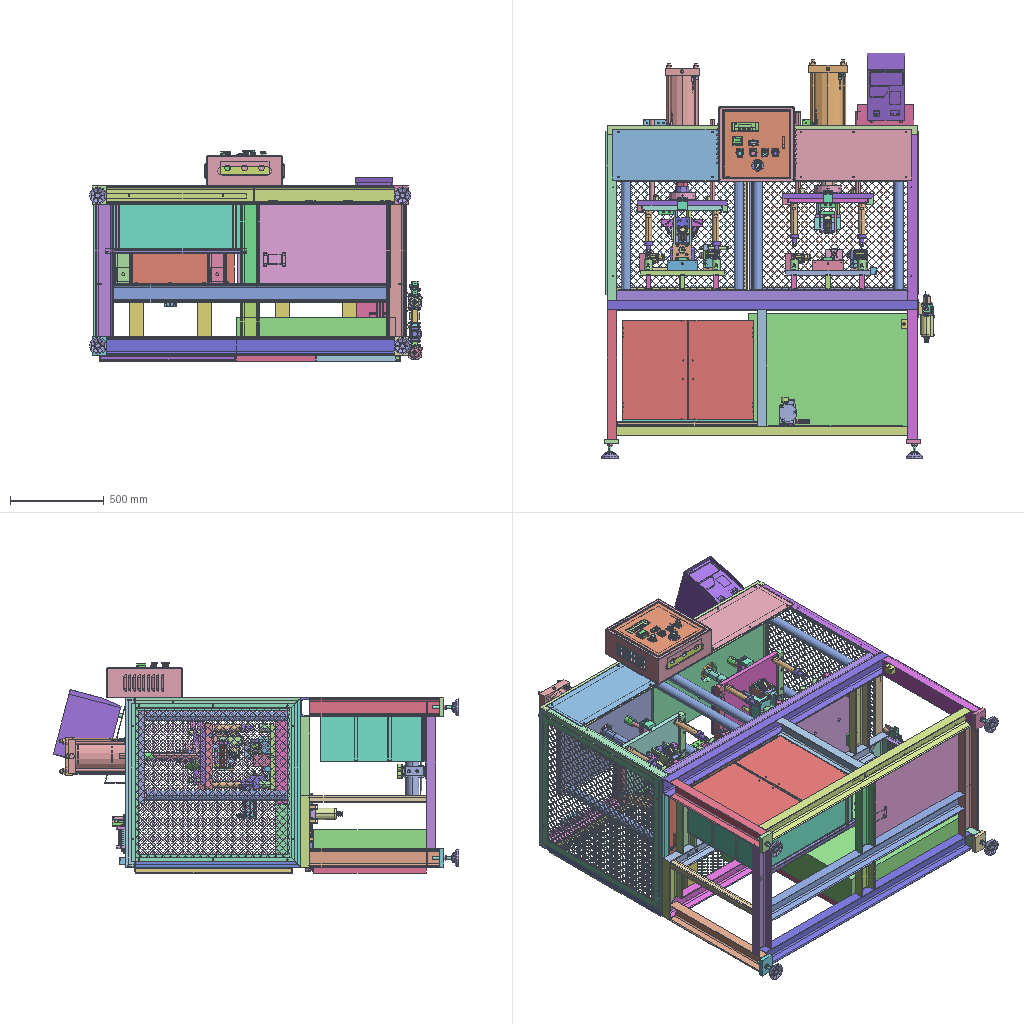Assembly | STEP file | 178 different items | 377 placed | box 1770 x 2157 x 1125 mm
Parts list (item | name | quantity | parent item | size | volume):
1 | CDS1FN160-250-A54Z_CS1-Body-1 | x1 | in CDS1FN160-250-A54Z | 182 x 182 x 425 mm | 4151915 mm3
2 | CDS1FN160-250-A54Z_CS1-Rod | x2 | in CDS1FN160-250-A54Z | 160 x 160 x 425.5 mm | 614336 mm3
3 | CDS1FN160-250-A54Z_CS1-Flange | x1 | in CDS1FN160-250-A54Z | 275 x 180 x 20 mm | 823998 mm3
4 | CDS1FN160-250-A54Z_A5_A6_F5_J5_ForLargeBore | x2 | in CDS1FN160-250-A54Z | 32 x 26 x 89 mm | 7994 mm3
5 | CDS1FN180-250-A54Z_CS1-Rod | x2 | in CDS1FN180-250-A54Z | 180 x 180 x 445 mm | 804374 mm3
6 | CDS1FN180-250-A54Z_CS1-Body-1 | x1 | in CDS1FN180-250-A54Z | 204 x 204 x 444 mm | 5555129 mm3
7 | CDS1FN180-250-A54Z_CS1-Flange | x1 | in CDS1FN180-250-A54Z | 320 x 200 x 25 mm | 1269642 mm3
8 | CDS1FN180-250-A54Z_A5_A6_F5_J5_ForLargeBore | x2 | in CDS1FN180-250-A54Z | 34 x 28 x 89 mm | 8233 mm3
9 | NT-16_CS1-RodEndNut | x1 | in NT-16 | 55 x 63.509 x 21 mm | 33434 mm3
10 | NT-18_Nuts | x1 | in NT-18 | 60.016 x 69.3 x 23 mm | 42288 mm3
11 | CQ2B40-30D_CQ2Tube | x4 | in CQ2B40-30D, CQ2B40-30D-1, CQ2B40-30D-2, CQ2B40-30D-3 | 52 x 57 x 59.5 mm | 79624 mm3
12 | CQ2B40-30D_CQ22031Rods | x4 | in CQ2B40-30D, CQ2B40-30D-1, CQ2B40-30D-2, CQ2B40-30D-3 | 40 x 40 x 54.25 mm | 15444 mm3
13 | CQ2B40-30D_CQ2 SnapRing | x4 | in CQ2B40-30D, CQ2B40-30D-1, CQ2B40-30D-2, CQ2B40-30D-3 | 44.5 x 43.888 x 7 mm | 5046 mm3
14 | HANYOUNG CR-253 5A | x2 | in Assy Hanyoung CR-253, panel box 500 x 600 x 200 | 32.5 x 45.5 x 64.5 mm | 42497 mm3
15 | Switch CR-253 | x1 | in Assy Hanyoung CR-253 | 24 x 35.897 x 23 mm | 7467 mm3
16 | B18.6.7M - M3 x 0.5 x 5 Type I Cross Recessed PHMS --5N | x8 | in Assy Hanyoung CR-253, Assy H7EC | 7.373 x 5.6 x 5.6 mm | 81.485 mm3
17 | OMRON H7EC | x1 | in Assy H7EC | 47.6 x 23.8 x 55.5 mm | 8164 mm3
18 | B18.6.7M - M4 x 0.7 x 5 Type I Cross Recessed PHMS --5N | x4 | in Assy H7EC | 8.067 x 8 x 8 mm | 178.262 mm3
19 | Cover | x1 | in Assy H7EC | 48 x 35 x 26.5 mm | 5852 mm3
20 | Karet | x1 | in Assy H7EC | 50 x 27 x 2.5 mm | 725.773 mm3
21 | Omron | x1 | in COUNTER OMRON | 109 x 47.8 x 53.73 mm | 203116 mm3
22 | panel body | x1 | in panel box 500 x 600 x 200 | 424 x 400 x 160 mm | 948430 mm3
23 | panel body dalam | x1 | in panel box 500 x 600 x 200 | 300 x 300 x 10 mm | 177458 mm3
24 | tutup bawah | x1 | in panel box 500 x 600 x 200 | 260 x 1.8 x 70 mm | 28943 mm3
25 | panel body depan | x1 | in panel box 500 x 600 x 200 | 352 x 381.4 x 22.754 mm | 281354 mm3
26 | Vexta Operation Unit OP200A | x1 | in panel box 500 x 600 x 200 | 142 x 48 x 17.4 mm | 105973 mm3
27 | Emergency hanyoung | x1 | in panel box 500 x 600 x 200 | 39.095 x 47.049 x 74 mm | 39082 mm3
28 | push_lamp1 | x1 | in panel box 500 x 600 x 200 | 36 x 54.3 x 68.1 mm | 76407 mm3
29 | Fuji Electric AR9T511-M | x1 | in panel box 500 x 600 x 200 | 30 x 39.5 x 78 mm | 61141 mm3
30 | Emergency Label | x1 | in panel box 500 x 600 x 200 | 64 x 1 x 64 mm | 2571 mm3
31 | Legend Standby | x4 | in panel box 500 x 600 x 200 | 41.068 x 43.269 x 1.43 mm | 1005 mm3
32 | CQ2A50-125DC-R06US_AS3054 Body | x2 | in CQ2A50-125DC-R06US_AS3054, CQ2A50-125DC-R06US_AS3054-1 | 34.45 x 40.4 x 19.63 mm | 8086 mm3
33 | CQ2A50-125DC-R06US_CQ2Tube | x1 | in CQ2A50-125DC-R06US | 64 x 71 x 180.5 mm | 380542 mm3
34 | CQ2A50-125DC-R06US_CQ22031Rods | x1 | in CQ2A50-125DC-R06US | 50 x 50 x 173.25 mm | 61293 mm3
35 | CQ2A50-125DC-R06US_CQ2 SnapRing | x1 | in CQ2A50-125DC-R06US | 55 x 54.243 x 13.3 mm | 12652 mm3
36 | AC10B-M5_AC3011A Spacer Interface(1) | x1 | in AC10B-M5_AC3011A Spacer(100T) | 6 x 25.75 x 33 mm | 2218 mm3
37 | AC10B-M5_AC3011A Spacer Front Plate(1) | x1 | in AC10B-M5_AC3011A Spacer(100T) | 13.502 x 24.5 x 7.058 mm | 480.167 mm3
38 | AC10B-M5_AC3011A AF Bowl(10)-1 | x1 | in AC10B-M5_AC3011A AF Bowl Assy(10) | 26.2 x 41.1 x 26.2 mm | 3344 mm3
39 | AC10B-M5_AC3011A AF Drain(10)-1 | x1 | in AC10B-M5_AC3011A AF Bowl Assy(10) | 11.5 x 8.4 x 11.5 mm | 268.613 mm3
40 | AC10B-M5_AC3011A AF Body(10)-1 | x1 | in AC10B-M5 | 25 x 17.5 x 25 mm | 8195 mm3
41 | AC10B-M5_AC3011A AR Body(10)-1 | x1 | in AC10B-M5 | 25 x 58 x 25 mm | 17859 mm3
42 | AC10B-M5_AC3011A Plug(00) | x2 | in AC10B-M5 | 6.85 x 8.115 x 8.115 mm | 313.171 mm3
43 | Cosmo LS-1862 | x1 | in 43 | 198 x 303.553 x 384.993 mm | 18480942 mm3
44 | SS5V1-16S3AD-08B-N1_CAInput Side End Plate | x1 | in SS5V1-16S3AD-08B-N1_EX120 Connector Block | 30 x 67.2 x 95.55 mm | 93320 mm3
45 | SS5V1-16S3AD-08B-N1_Rail Clamp | x2 | in SS5V1-16S3AD-08B-N1_EX120 Connector Block, SS5V1-16S3AD-08B-N1_CAExhaust Side | 11 x 10 x 87 mm | 2335 mm3
46 | SS5V1-16S3AD-08B-N1_Exhaust Cap | x2 | in SS5V1-16S3AD-08B-N1_EX120 Connector Block, SS5V1-16S3AD-08B-N1_CAExhaust Side | 16.5 x 8.5 x 63 mm | 8670 mm3
47 | SS5V1-16S3AD-08B-N1_SV Fittings | x4 | in SS5V1-16S3AD-08B-N1_EX120 Connector Block, SS5V1-16S3AD-08B-N1_CAExhaust Side | 14 x 14 x 19.5 mm | 1887 mm3
48 | SS5V1-16S3AD-08B-N1_EX120 Adapter | x1 | in SS5V1-16S3AD-08B-N1_EX120 Connector Block | 68.5 x 61 x 26.75 mm | 64315 mm3
49 | SS5V1-16S3AD-08B-N1_EX120 SI Unit | x1 | in SS5V1-16S3AD-08B-N1_EX120 Connector Block | 64 x 61 x 28.8 mm | 102624 mm3
50 | SS5V1-16S3AD-08B-N1_Valve Base | x8 | in SS5V1-16S3AD-08B-N1_Base, SS5V1-16S3AD-08B-N1_Base-1, SS5V1-16S3AD-08B-N1_Base-2, SS5V1-16S3AD-08B-N1_Base-3, SS5V1-16S3AD-08B-N1_Base-4, SS5V1-16S3AD-08B-N1_Base-5, SS5V1-16S3AD-08B-N1_Base-6, SS5V1-16S3AD-08B-N1_Base-7 | 10.5 x 34 x 95.55 mm | 27614 mm3
51 | SS5V1-16S3AD-08B-N1_VV5Q Fittings | x16 | in SS5V1-16S3AD-08B-N1_Base, SS5V1-16S3AD-08B-N1_Base-1, SS5V1-16S3AD-08B-N1_Base-2, SS5V1-16S3AD-08B-N1_Base-3, SS5V1-16S3AD-08B-N1_Base-4, SS5V1-16S3AD-08B-N1_Base-5, SS5V1-16S3AD-08B-N1_Base-6, SS5V1-16S3AD-08B-N1_Base-7 | 10 x 10 x 16 mm | 989.757 mm3
52 | SS5V1-16S3AD-08B-N1_CAD Side End Plate | x1 | in SS5V1-16S3AD-08B-N1_CAExhaust Side | 30.5 x 38.5 x 95.55 mm | 62940 mm3
53 | SS5V1-16S3AD-08B-N1_AXT100-DR | x1 | in SS5V1-16S3AD-08B-N1 | 35 x 7.5 x 210.5 mm | 13884 mm3
54 | VBA22A-03GN_AN6009 Silencer | x1 | in VBA22A-03GN_AN6009 | 25.403 x 84 x 25 mm | 9196 mm3
55 | VBA22A-03GN_VBA20A Body | x1 | in VBA22A-03GN | 300 x 127.5 x 92.8 mm | 1446394 mm3
56 | VBA22A-03GN_G36-10-N01 | x2 | in VBA22A-03GN | 37 x 41.5 x 37 mm | 27826 mm3
57 | VBA22A-03GN_VBA20A Bracket | x1 | in VBA22A-03GN | 118 x 11 x 73 mm | 25260 mm3
58 | AC40-04-KSTV-38JNR_AC3009A Spacer Interface | x6 | in AC40-04-KSTV-38JNR_AC3009A Spacer(400T-R), AC40-04-KSTV-38JNR_AC3009A Spacer(400-R), AC40-04-KSTV-38JNR_AC3009A Spacer(400T-R)-1, AC40-04-KSTV-38JNR_AC3009A Spacer(400-R)-1, AC40-04-KSTV-38JNR_AC3009A Spacer(400T-R)-2, AC40-04-KSTV-38JNR_AC3009A Spacer(400T-R)-3 | 9 x 56.65 x 65 mm | 9428 mm3
59 | AC40-04-KSTV-38JNR_AC3009A Spacer Rear Plate(4T) | x4 | in AC40-04-KSTV-38JNR_AC3009A Spacer(400T-R), AC40-04-KSTV-38JNR_AC3009A Spacer(400T-R)-1, AC40-04-KSTV-38JNR_AC3009A Spacer(400T-R)-2, AC40-04-KSTV-38JNR_AC3009A Spacer(400T-R)-3 | 26 x 96 x 34.173 mm | 17760 mm3
60 | AC40-04-KSTV-38JNR_AC3009A Spacer Front Plate | x6 | in AC40-04-KSTV-38JNR_AC3009A Spacer(400T-R), AC40-04-KSTV-38JNR_AC3009A Spacer(400-R), AC40-04-KSTV-38JNR_AC3009A Spacer(400T-R)-1, AC40-04-KSTV-38JNR_AC3009A Spacer(400-R)-1, AC40-04-KSTV-38JNR_AC3009A Spacer(400T-R)-2, AC40-04-KSTV-38JNR_AC3009A Spacer(400T-R)-3 | 18.505 x 54.2 x 10.913 mm | 2347 mm3
61 | AC40-04-KSTV-38JNR_AC3009A Spacer Rear Plate(4) | x2 | in AC40-04-KSTV-38JNR_AC3009A Spacer(400-R), AC40-04-KSTV-38JNR_AC3009A Spacer(400-R)-1 | 18.951 x 54 x 7.773 mm | 1709 mm3
62 | AC40-04-KSTV-38JNR_AC3009A AF Bowl-2 | x1 | in AC40-04-KSTV-38JNR_AC3009A AF Bowl Assy | 61.5 x 121.9 x 71.711 mm | 50188 mm3
63 | AC40-04-KSTV-38JNR_AC3009A AF Drain-2 | x1 | in AC40-04-KSTV-38JNR_AC3009A AF Bowl Assy | 19.63 x 18.1 x 17 mm | 2625 mm3
64 | AC40-04-KSTV-38JNR_AC3009A AL Bowl-2 | x1 | in AC40-04-KSTV-38JNR_AC3009A AL Bowl Assy | 61.5 x 121.9 x 71.711 mm | 50188 mm3
65 | AC40-04-KSTV-38JNR_AC3009A AL Drain-2 | x1 | in AC40-04-KSTV-38JNR_AC3009A AL Bowl Assy | 28 x 24.1 x 28 mm | 7214 mm3
66 | AC40-04-KSTV-38JNR_AC3009A VHS Body-1 | x1 | in AC40-04-KSTV-38JNR_AC3009A VHS | 70 x 60.6 x 58 mm | 70876 mm3
67 | AC40-04-KSTV-38JNR_AC3009A VHS Handle | x1 | in AC40-04-KSTV-38JNR_AC3009A VHS | 63 x 46.4 x 58 mm | 68850 mm3
68 | AC40-04-KSTV-38JNR_AC3009A AR Body-1 | x1 | in AC40-04-KSTV-38JNR | 70 x 128 x 57.6 mm | 240174 mm3
69 | AC40-04-KSTV-38JNR_AC3009A T Interface-1 | x1 | in AC40-04-KSTV-38JNR | 24 x 62 x 36 mm | 21819 mm3
70 | AC40-04-KSTV-38JNR_AC3009A AF Body-1 | x1 | in AC40-04-KSTV-38JNR | 70 x 52 x 70 mm | 171815 mm3
71 | AC40-04-KSTV-38JNR_AC3009A Switch | x1 | in AC40-04-KSTV-38JNR | 15 x 111 x 36 mm | 31675 mm3
72 | AC40-04-KSTV-38JNR_AC3009A AKM Body | x1 | in AC40-04-KSTV-38JNR | 70 x 42 x 54 mm | 78893 mm3
73 | AC40-04-KSTV-38JNR_AC3009A AL Body-1 | x1 | in AC40-04-KSTV-38JNR | 70 x 74 x 70 mm | 184515 mm3
74 | AC40-04-KSTV-38JNR_AC3009A Gauge-2 | x1 | in AC40-04-KSTV-38JNR | 28 x 28 x 5 mm | 3081 mm3
75 | AC40-04-KSTV-38JNR_AC3009A Plug | x1 | in AC40-04-KSTV-38JNR | 10.8 x 13.845 x 13.845 mm | 1426 mm3
76 | OP10-001_base frame(Default_As Machined_) | x1 | - | 1680 x 792 x 900 mm | 25499684 mm3
77 | OP10-002_upper frame(Default_As Machined_) | x1 | - | 1650 x 1042 x 900 mm | 8540478 mm3
78 | OP10-003_front cover (R) | x1 | - | 620 x 5 x 270 mm | 835492 mm3
79 | OP10-004_front cover (L) | x1 | - | 560 x 5 x 270 mm | 754995 mm3
80 | OP10-005_side cover | x2 | - | - | 1174721 mm3
81 | OP10-006_rear cover (R) | x1 | - | - | 1354437 mm3
82 | OP10-007_rear cover (L) | x1 | - | - | 1150842 mm3
83 | OP10-009_shelf(Default_As Machined_) | x1 | - | 750 x 565 x 320 mm | 3649347 mm3
84 | OP10-010_junction block (A) | x2 | - | 220 x 35 x 35 mm | 246704 mm3
85 | OP10-011_junction block (B) | x1 | - | 190 x 35 x 35 mm | 212721 mm3
86 | OP10-012_junction block (C) | x1 | - | 130 x 35 x 35 mm | 144755 mm3
87 | OP10-013_junction block (D) | x1 | - | 50 x 35 x 35 mm | 54198 mm3
88 | OP10-014_lower plate (R) | x1 | - | 830 x 30 x 500 mm | 12317635 mm3
89 | OP10-015_upper plate (R) | x1 | - | 830 x 30 x 500 mm | 11965726 mm3
90 | OP10-016_lower plate (L)  | x1 | - | 680 x 30 x 500 mm | 10067635 mm3
91 | OP10-017_upper plate (L) | x1 | - | 680 x 30 x 500 mm | 9842603 mm3
92 | OP10-018_base rib (A) | x2 | - | 25 x 75 x 500 mm | 930693 mm3
93 | OP10-019_base rib (B) | x4 | - | 25 x 75 x 500 mm | 929254 mm3
94 | OP10-020_central plate | x2 | - | 480 x 25 x 300 mm | 3542194 mm3
95 | OP10-021_guide(1) | x2 | - | 35 x 35 x 350 mm | 297564 mm3
96 | OP10-022_guide(2) | x2 | - | 35 x 35 x 350 mm | 297564 mm3
97 | OP10-023_clamp | x8 | - | 35 x 12 x 19 mm | 6394 mm3
98 | OP10-024_fix-pin | x4 | - | 25 x 72 x 25 mm | 20386 mm3
99 | OP10-025_stopper base | x2 | - | 65 x 28 x 50 mm | 72632 mm3
100 | OP10-026_stopper plate | x2 | - | 65 x 20 x 50 mm | 54932 mm3
101 | OP10-027_cylinder connector (R) | x1 | - | 70 x 85 x 85 mm | 228647 mm3
102 | OP10-028_cylinder connector (L) | x1 | - | 75 x 85 x 85 mm | 251301 mm3
103 | OP10-029_setting flange | x2 | - | 139.943 x 36 x 140 mm | 309110 mm3
104 | OP10-030_plate | x2 | - | 140 x 5 x 140 mm | 72351 mm3
105 | OP10-031_guide base | x4 | - | 250 x 22 x 75 mm | 400090 mm3
106 | OP10-032_collar | x8 | - | 30 x 13 x 30 mm | 7922 mm3
107 | OP10-033_setup guide  | x4 | - | 25 x 100 x 300 mm | 745616 mm3
108 | OP10-034_shelf-door | x2 | - | 530 x 5 x 345 mm | 913394 mm3
109 | OP10-101_base plate lower (R) | x1 | - | 450 x 25 x 350 mm | 3845451 mm3
110 | OP10-102_base plate lower (L) | x1 | - | 450 x 25 x 350 mm | 3834229 mm3
111 | OP10-104_upper base plate (R) | x1 | - | 430 x 25 x 350 mm | 3618986 mm3
112 | OP10-105_upper base plate (L)  | x1 | - | 430 x 25 x 350 mm | 3617980 mm3
113 | OP10-106_guide post | x8 | - | 35 x 178 x 35 mm | 152676 mm3
114 | OP10-107_guide-pin | x8 | - | 44 x 44 x 91 mm | 50039 mm3
115 | OP10-108_guide catch | x8 | - | 44 x 44 x 84 mm | 74087 mm3
116 | OP10-109_base block (lower)-R | x1 | - | 160 x 50 x 160 mm | 1246879 mm3
117 | OP10-111_base block (lower)-L  | x1 | - | 160 x 50 x 160 mm | 1248387 mm3
118 | OP10-113_round-pin | x2 | - | 12 x 12 x 27.5 mm | 2777 mm3
119 | OP10-114_dia-pin | x2 | - | 12 x 12 x 27.5 mm | 2777 mm3
120 | OP10-116_work-guide | x2 | - | 14 x 20 x 70 mm | 17393 mm3
121 | OP10-118_cylinder base (1) | x3 | - | 86 x 13 x 69 mm | 65313 mm3
122 | OP10-119_cylinder stand (1) -R | x1 | - | 86 x 13 x 94 mm | 86706 mm3
123 | OP10-120_cylinder stand (1) -L | x1 | - | 86 x 13 x 94 mm | 86098 mm3
124 | OP10-121_cylinder stand (2) -R | x1 | - | 86 x 13 x 98 mm | 98029 mm3
125 | OP10-122_rib plate | x6 | - | 13 x 50 x 56 mm | 32347 mm3
126 | OP10-123_seal rod | x4 | - | 31 x 38 x 31 mm | 15633 mm3
127 | OP10-124_seal pad | x4 | - | 31 x 10 x 31 mm | 7003 mm3
128 | OP10-125_seal rod dia7 | x1 | - | 20 x 38 x 20 mm | 6478 mm3
129 | OP10-126_seal pad dia7 | x1 | - | 14 x 10 x 14 mm | 1539 mm3
130 | OP10-127_cylinder base M6 | x1 | - | 30 x 30 x 80 mm | 45481 mm3
131 | OP10-128_seal head M6 | x1 | - | 16 x 18 x 16 mm | 2771 mm3
132 | OP10-129_seal pad M6 | x1 | - | 11 x 10 x 11 mm | 950.332 mm3
133 | OP10-130_cylinder base (2)-L | x1 | - | 128 x 20 x 70 mm | 155973 mm3
134 | OP10-131_cylinder stand (2) -L | x1 | - | 100 x 20 x 125 mm | 216562 mm3
135 | OP10-132_side plate (2)-L | x2 | - | 100 x 14 x 70 mm | 92004 mm3
136 | OP10-133_seal rod camshaft | x1 | - | 31 x 40 x 31 mm | 16299 mm3
137 | OP10-134_cylinder stand (3) | x2 | - | 88 x 38 x 60 mm | 176864 mm3
138 | OP10-135_junction block (E) | x1 | - | 170 x 35 x 35 mm | 190983 mm3
139 | OP10-136_junction block (F) | x1 | - | 200 x 35 x 35 mm | 224966 mm3
140 | OP10-137_base block (upper)-R | x1 | - | 130 x 20 x 130 mm | 318432 mm3
141 | OP10-139_base plate (F)-R | x1 | - | 72 x 14 x 100 mm | 94613 mm3
142 | OP10-140_side plate (F)-R | x2 | - | 10 x 48 x 110 mm | 45630 mm3
143 | OP10-141_inclined plate (F) | x2 | - | 72 x 14 x 58 mm | 45441 mm3
144 | OP10-142_seal rod plug | x2 | - | 22 x 38 x 22 mm | 7650 mm3
145 | OP10-143_seal pad plug | x2 | - | 16 x 10 x 16 mm | 2011 mm3
146 | OP10-144_upper seal block | x1 | - | 130 x 59.5 x 135 mm | 671635 mm3
147 | OP10-146_seal side plate (1) | x1 | - | 44 x 10 x 72 mm | 28330 mm3
148 | OP10-147_seal side plate (2) | x1 | - | 22 x 12 x 44 mm | 7394 mm3
149 | OP10-148_seal block | x1 | - | 25.2 x 15 x 49 mm | 13850 mm3
150 | OP10-149_base block (upper)-L | x1 | - | 106 x 20 x 130 mm | 253956 mm3
151 | OP10-150_clamp rod (L) | x2 | - | 18 x 48.5 x 18 mm | 11527 mm3
152 | OP10-151_seal rod (L) | x2 | - | 20 x 48.5 x 20 mm | 14002 mm3
153 | OP10-152_side plate upper-L1 | x1 | - | 12 x 40 x 218 mm | 95136 mm3
154 | OP10-153_side plate upper-L2 | x1 | - | 12 x 40 x 218 mm | 95136 mm3
155 | OP10-154_inclined plate (L) | x2 | - | 130 x 16 x 54 mm | 106815 mm3
156 | OP10-155_base plate (F)-L | x1 | - | 72 x 15 x 60 mm | 59226 mm3
157 | OP10-156_side plate (F)-L | x2 | - | 10 x 48 x 140 mm | 48244 mm3
158 | OP10-157_seal rod (valve guide) | x2 | - | 25 x 32 x 25 mm | 5292 mm3
159 | OP10-158_seal pad (valve guide) | x2 | - | 20 x 18 x 20 mm | 4188 mm3
160 | OP10-159_seal block (2nd air pass) | x1 | - | 75 x 28 x 64 mm | 36277 mm3
161 | OP10-160_seal pad (2nd air pass) | x1 | - | 14 x 10 x 14 mm | 981.355 mm3
162 | OP10-161_junction block (G) | x2 | - | 80 x 25 x 25 mm | 42075 mm3
163 | circular post SPCD-SSB-D50-L760-E5-P30-M16-F15-V30-MA16-SC40-W20-S41 | x8 | - | 50 x 50 x 780 mm | 1506737 mm3
164 | socket head cap screw_iso(ISO 4762 M16 x 35 --- 35N) | x8 | - | 51 x 24 x 24 mm | 12641 mm3
165 | plain washer small grade a_iso(Washer ISO 7092 - 20) | x8 | - | 3 x 34 x 34 mm | 1685 mm3
166 | hex screw gradec_iso(ISO 4018 - M6 x 25-WN) | x1 | - | 29.375 x 11.547 x 10 mm | 1078 mm3
167 | hex nut gradec_iso(Hexagon Nut ISO - 4034 - M6 - N) | x1 | - | 10 x 11.547 x 6.1 mm | 403.17 mm3
168 | Air Cylinder CQ2B32-30D | x1 | - | 45.2 x 49.7 x 50 mm | 69030 mm3
169 | Control Box | x1 | - | 235 x 600 x 850 mm | 117277509 mm3
170 | hex thin nut gradeb_iso(Hexagon Nut ISO - 4036 - M8 - N) | x4 | - | 13 x 15.011 x 4 mm | 434.11 mm3
171 | CDJ2B16-75-B | x1 | - | 18.4 x 18.4 x 150.2 mm | 31123 mm3
172 | Air Cylinder CQ2B32-50D | x2 | - | 45.2 x 49.7 x 70 mm | 103939 mm3
173 | Air Cylinder CQ2B20-30DC | x2 | - | 54.5 x 36 x 36 mm | 48635 mm3
174 | slide bush dia25 | x4 | - | 62 x 120 x 62 mm | 123111 mm3
175 | slide shaft dia25x440 | x4 | - | 25 x 440 x 25 mm | 213800 mm3
176 | circular post spca dia22-16-M8 | x4 | - | 22 x 59.7 x 22 mm | 21361 mm3
177 | circular post dia22-16-M8 | x4 | - | 22 x 71.7 x 22 mm | 23541 mm3
178 | Foot ACOMPANY_AD16_100e | x4 | - | - | -
Placements (level | parent | child | x y z in mm | rotation matrix by rows), first 257 of 419 lines:
1 | subassembly 2 | CDS1FN160-250-A54Z | -450.446 1409.374 163.364 | 0 -1 0 0 0 -1 1 0 0
2 | CDS1FN160-250-A54Z | CDS1FN160-250-A54Z_CS1-Body-1 | -0.0 -0.0 -0.0 | 1 0 0 0 1 0 0 0 1
2 | CDS1FN160-250-A54Z | CDS1FN160-250-A54Z_CS1-Rod | -0.0 -0.0 -127.5 | 1 0 0 0 1 0 0 0 1
2 | CDS1FN160-250-A54Z | CDS1FN160-250-A54Z_CS1-Flange | -0.0 -0.0 188.0 | 1 0 0 0 1 0 0 0 1
2 | CDS1FN160-250-A54Z | CDS1FN160-250-A54Z_A5_A6_F5_J5_ForLargeBore | 77.0 56.0 106.0 | 0 1 0 -1 0 0 0 0 1
2 | CDS1FN160-250-A54Z | CDS1FN160-250-A54Z_A5_A6_F5_J5_ForLargeBore | 77.0 -56.0 -106.0 | 0 1 0 1 0 0 0 0 -1
1 | subassembly 2 | CDS1FN180-250-A54Z | 324.554 1418.874 163.364 | 0 -1 0 0 0 -1 1 0 0
2 | CDS1FN180-250-A54Z | CDS1FN180-250-A54Z_CS1-Rod | -0.0 -0.0 -127.5 | 1 0 0 0 1 0 0 0 1
2 | CDS1FN180-250-A54Z | CDS1FN180-250-A54Z_CS1-Body-1 | -0.0 -0.0 -0.0 | 1 0 0 0 1 0 0 0 1
2 | CDS1FN180-250-A54Z | CDS1FN180-250-A54Z_CS1-Flange | -0.0 -0.0 195.0 | 1 0 0 0 1 0 0 0 1
2 | CDS1FN180-250-A54Z | CDS1FN180-250-A54Z_A5_A6_F5_J5_ForLargeBore | 87.0 -64.0 -109.0 | 0 1 0 1 0 0 0 0 -1
2 | CDS1FN180-250-A54Z | CDS1FN180-250-A54Z_A5_A6_F5_J5_ForLargeBore | 87.0 64.0 107.0 | 0 1 0 -1 0 0 0 0 1
1 | subassembly 2 | NT-16 | -450.446 967.455 163.364 | 0.9845 -0.1755 0 0 0 1 -0.1755 -0.9845 0
2 | NT-16 | NT-16_CS1-RodEndNut | -0.0 -0.0 -0.0 | 1 0 0 0 1 0 0 0 1
1 | subassembly 2 | NT-18 | 324.554 1001.861 163.364 | -0.07623 -0.9971 0 0 0 1 -0.9971 0.07623 0
2 | NT-18 | NT-18_Nuts | -0.0 -0.0 -0.0 | 1 0 0 0 1 0 0 0 1
1 | subassembly 2 | CQ2B40-30D | 498.22 591.374 221.187 | -0.2594 0 -0.9658 0 1 0 0.9658 0 -0.2594
2 | CQ2B40-30D | CQ2B40-30D_CQ2Tube | -0.0 -0.0 -0.0 | 1 0 0 0 1 0 0 0 1
2 | CQ2B40-30D | CQ2B40-30D_CQ22031Rods | -0.0 -0.0 -17.5 | 1 0 0 0 1 0 0 0 1
2 | CQ2B40-30D | CQ2B40-30D_CQ2 SnapRing | -0.0 0.0 24.15 | 1 0 0 0 1 0 0 0 1
1 | subassembly 2 | CQ2B40-30D-1 | -286.218 591.374 202.972 | -0.2594 0 -0.9658 0 1 0 0.9658 0 -0.2594
2 | CQ2B40-30D-1 | CQ2B40-30D_CQ2Tube | -0.0 -0.0 -0.0 | 1 0 0 0 1 0 0 0 1
2 | CQ2B40-30D-1 | CQ2B40-30D_CQ22031Rods | -0.0 0.0 -17.5 | 1 0 0 0 1 0 0 0 1
2 | CQ2B40-30D-1 | CQ2B40-30D_CQ2 SnapRing | -0.0 0.0 24.15 | 1 0 0 0 1 0 0 0 1
1 | subassembly 2 | panel box 500 x 600 x 200 | -55.446 1181.374 473.364 | 1 0 0 0 1 0 0 0 1
2 | panel box 500 x 600 x 200 | Assy Hanyoung CR-253 | 55.471 -45.761 147.79 | -1 0 0 0 -1 0 0 0 1
3 | Assy Hanyoung CR-253 | HANYOUNG CR-253 5A | 11.192 2.931 10.41 | 1 0 0 0 1 0 0 0 1
3 | Assy Hanyoung CR-253 | Switch CR-253 | 11.192 2.931 19.41 | 0.8204 0.5718 0 -0.5718 0.8204 0 0 0 1
3 | Assy Hanyoung CR-253 | B18.6.7M - M3 x 0.5 x 5 Type I Cross Recessed PHMS --5N | 20.192 -19.819 -30.49 | 0 0 -1 0 1 0 1 0 -0
3 | Assy Hanyoung CR-253 | B18.6.7M - M3 x 0.5 x 5 Type I Cross Recessed PHMS --5N | 23.067 -1.561 -15.49 | 0 0 -1 0 1 0 1 0 -0
3 | Assy Hanyoung CR-253 | B18.6.7M - M3 x 0.5 x 5 Type I Cross Recessed PHMS --5N | -0.6828 -1.561 -15.49 | 0 0 -1 0 1 0 1 0 -0
3 | Assy Hanyoung CR-253 | B18.6.7M - M3 x 0.5 x 5 Type I Cross Recessed PHMS --5N | 2.192 -21.69 -11.114 | 0 -0.7071 -0.7071 0.7071 0.5 -0.5 0.7071 -0.5 0.5
3 | Assy Hanyoung CR-253 | B18.6.7M - M3 x 0.5 x 5 Type I Cross Recessed PHMS --5N | 20.192 -21.69 -11.114 | 0 -0.7071 -0.7071 0.7071 0.5 -0.5 0.7071 -0.5 0.5
3 | Assy Hanyoung CR-253 | B18.6.7M - M3 x 0.5 x 5 Type I Cross Recessed PHMS --5N | 2.192 -19.819 -30.49 | 0 0 -1 0 1 0 1 0 -0
2 | panel box 500 x 600 x 200 | Assy H7EC | -25.552 6.462 147.044 | 1 0 0 0 1 0 0 0 1
3 | Assy H7EC | B18.6.7M - M3 x 0.5 x 5 Type I Cross Recessed PHMS --5N | 30.002 15.05 -11.79 | 0 0.5542 -0.8324 0 0.8324 0.5542 1 0 0
3 | Assy H7EC | B18.6.7M - M3 x 0.5 x 5 Type I Cross Recessed PHMS --5N | -11.998 -13.45 -11.79 | 0 -0.383 -0.9237 0 0.9237 -0.383 1 0 0
3 | Assy H7EC | OMRON H7EC | 9.002 0.8001 20.456 | 1 0 0 0 1 0 0 0 1
3 | Assy H7EC | B18.6.7M - M4 x 0.7 x 5 Type I Cross Recessed PHMS --5N | -8.248 0.8001 -29.144 | 0 0 -1 0 1 0 1 0 0
3 | Assy H7EC | B18.6.7M - M4 x 0.7 x 5 Type I Cross Recessed PHMS --5N | 0.752 0.8001 -29.144 | 0 0 -1 0 1 0 1 0 0
3 | Assy H7EC | B18.6.7M - M4 x 0.7 x 5 Type I Cross Recessed PHMS --5N | 17.252 0.8001 -29.144 | 0 0 -1 0 1 0 1 0 0
3 | Assy H7EC | B18.6.7M - M4 x 0.7 x 5 Type I Cross Recessed PHMS --5N | 26.252 0.8001 -29.144 | 0 0 -1 0 1 0 1 0 0
3 | Assy H7EC | Cover | 9.002 0.8001 -14.89 | -1 0 0 0 1 0 0 0 -1
3 | Assy H7EC | Karet | 9.002 0.8001 14.206 | 1 0 0 0 1 0 0 0 1
2 | panel box 500 x 600 x 200 | COUNTER OMRON | -117.575 22.398 144.407 | 0 0 -1 0 1 0 1 0 -0
3 | COUNTER OMRON | Omron | 36.593 -6.037 -15.208 | 1 0 0 0 1 0 0 0 1
2 | panel box 500 x 600 x 200 | panel body | -0.0 -0.0 -0.0 | 1 0 0 0 1 0 0 0 1
2 | panel box 500 x 600 x 200 | panel body dalam | 0.0 -0.0 31.8 | 1 0 0 0 1 0 0 0 1
2 | panel box 500 x 600 x 200 | tutup bawah | 0.0 -198.2 96.47 | 1 0 0 0 1 0 0 0 1
2 | panel box 500 x 600 x 200 | panel body depan | -0.0274 -0.0 158.2 | 1 0 0 0 1 0 0 0 1
2 | panel box 500 x 600 x 200 | HANYOUNG CR-253 5A | -17.938 -47.958 158.2 | 1 0 0 0 1 0 0 0 1
2 | panel box 500 x 600 x 200 | Vexta Operation Unit OP200A | -129.863 71.081 146.0 | 1 0 0 0 1 0 0 0 1
2 | panel box 500 x 600 x 200 | Emergency hanyoung | 6.599 -112.054 187.7 | 1 0 0 0 1 0 0 0 1
2 | panel box 500 x 600 x 200 | push_lamp1 | 82.119 -71.517 116.1 | 1 0 0 0 1 0 0 0 1
2 | panel box 500 x 600 x 200 | Fuji Electric AR9T511-M | -88.924 -49.355 158.2 | 1 0 0 0 1 0 0 0 1
2 | panel box 500 x 600 x 200 | Emergency Label | 6.599 -112.054 160.0 | 1 0 0 0 0 -1 0 1 0
2 | panel box 500 x 600 x 200 | Legend Standby | 71.213 -48.182 196.669 | 1 0 0 0 1 0 0 0 1
2 | panel box 500 x 600 x 200 | Legend Standby | -117.83 -48.67 196.669 | 1 0 0 0 1 0 0 0 1
2 | panel box 500 x 600 x 200 | Legend Standby | -46.843 -47.273 196.669 | 1 0 0 0 1 0 0 0 1
2 | panel box 500 x 600 x 200 | Legend Standby | 15.373 -48.006 196.669 | 1 0 0 0 1 0 0 0 1
1 | subassembly 2 | CQ2A50-125DC-R06US | -451.836 620.174 -75.886 | 1 0 0 0 1 0 0 0 1
2 | CQ2A50-125DC-R06US | CQ2A50-125DC-R06US_AS3054 | -0.0 51.2 76.25 | 1 0 0 0 1 0 0 0 1
3 | CQ2A50-125DC-R06US_AS3054 | CQ2A50-125DC-R06US_AS3054 Body | -0.0 -0.0 -0.0 | 1 0 0 0 1 0 0 0 1
2 | CQ2A50-125DC-R06US | CQ2A50-125DC-R06US_AS3054-1 | -0.0 51.2 -76.25 | 1 0 0 0 1 0 0 0 1
3 | CQ2A50-125DC-R06US_AS3054-1 | CQ2A50-125DC-R06US_AS3054 Body | -0.0 -0.0 -0.0 | 1 0 0 0 1 0 0 0 1
2 | CQ2A50-125DC-R06US | CQ2A50-125DC-R06US_CQ2Tube | -0.0 -0.0 -0.0 | 1 0 0 0 1 0 0 0 1
2 | CQ2A50-125DC-R06US | CQ2A50-125DC-R06US_CQ22031Rods | -0.0 -0.0 -65.0 | 1 0 0 0 1 0 0 0 1
2 | CQ2A50-125DC-R06US | CQ2A50-125DC-R06US_CQ2 SnapRing | -0.0 -0.0 84.45 | 1 0 0 0 1 0 0 0 1
1 | subassembly 2 | Cosmo LS-1862 | 626.603 1465.93 255.581 | 1 0 0 0 0.9673 -0.2537 0 0.2537 0.9673
2 | Cosmo LS-1862 | AC10B-M5 | 38.604 71.032 -163.233 | 0 0 -1 0 1 0 1 0 0
3 | AC10B-M5 | AC10B-M5_AC3011A Spacer(100T) | -0.0 0.0 -0.0 | 1 0 0 0 1 0 0 0 1
4 | AC10B-M5_AC3011A Spacer(100T) | AC10B-M5_AC3011A Spacer Interface(1) | 0.0 -0.0 -0.0 | 1 0 0 0 1 0 0 0 1
4 | AC10B-M5_AC3011A Spacer(100T) | AC10B-M5_AC3011A Spacer Front Plate(1) | 0.0 -0.0 12.8 | 1 0 0 0 1 0 0 0 1
3 | AC10B-M5 | AC10B-M5_AC3011A AF Bowl Assy(10) | -15.5 -10.5 -0.0 | 1 0 0 0 1 0 0 0 1
4 | AC10B-M5_AC3011A AF Bowl Assy(10) | AC10B-M5_AC3011A AF Bowl(10)-1 | -0.0 -0.0 -0.0 | 1 0 0 0 1 0 0 0 1
4 | AC10B-M5_AC3011A AF Bowl Assy(10) | AC10B-M5_AC3011A AF Drain(10)-1 | 0.0 -41.1 -0.0 | 1 0 0 0 1 0 0 0 1
3 | AC10B-M5 | AC10B-M5_AC3011A AF Body(10)-1 | -15.5 0.0 -0.0 | 1 0 0 0 1 0 0 0 1
3 | AC10B-M5 | AC10B-M5_AC3011A AR Body(10)-1 | 15.5 0.0 -0.0 | 1 0 0 0 1 0 0 0 1
3 | AC10B-M5 | AC10B-M5_AC3011A Plug(00) | 15.5 0.0 13.0 | 0 0 1 0 1 0 -1 0 0
3 | AC10B-M5 | AC10B-M5_AC3011A Plug(00) | 15.5 -3.3 -13.0 | 0 0 1 0 -1 0 1 0 -0
2 | Cosmo LS-1862 | Cosmo LS-1862 | 6.534 -399.184 267.752 | 1 0 0 0 1 0 0 0 1
1 | subassembly 2 | CQ2B40-30D-2 | -610.617 574.983 151.791 | 0.08579 0.176 0.9806 -0.9962 0 0.08716 0.01534 -0.9844 0.1754
2 | CQ2B40-30D-2 | CQ2B40-30D_CQ2Tube | -0.0 -0.0 -0.0 | 1 0 0 0 1 0 0 0 1
2 | CQ2B40-30D-2 | CQ2B40-30D_CQ22031Rods | -0.0 0.0 -17.5 | 1 0 0 0 1 0 0 0 1
2 | CQ2B40-30D-2 | CQ2B40-30D_CQ2 SnapRing | 0.0 0.0 24.15 | 1 0 0 0 1 0 0 0 1
1 | subassembly 2 | CQ2B40-30D-3 | 164.381 574.983 151.789 | 0.08579 0.176 0.9806 -0.9962 0 0.08716 0.01534 -0.9844 0.1754
2 | CQ2B40-30D-3 | CQ2B40-30D_CQ2Tube | -0.0 -0.0 -0.0 | 1 0 0 0 1 0 0 0 1
2 | CQ2B40-30D-3 | CQ2B40-30D_CQ22031Rods | -0.0 0.0 -17.5 | 1 0 0 0 1 0 0 0 1
2 | CQ2B40-30D-3 | CQ2B40-30D_CQ2 SnapRing | 0.0 0.0 24.15 | 1 0 0 0 1 0 0 0 1
1 | subassembly 2 | SS5V1-16S3AD-08B-N1 | 665.582 1284.674 -228.723 | 0 0 1 0 1 0 -1 0 0
2 | SS5V1-16S3AD-08B-N1 | SS5V1-16S3AD-08B-N1_EX120 Connector Block | -0.0 -0.0 -0.0 | 1 0 0 0 1 0 0 0 1
3 | SS5V1-16S3AD-08B-N1_EX120 Connector Block | SS5V1-16S3AD-08B-N1_CAInput Side End Plate | -8.4 19.25 -10.75 | 1 0 0 0 1 0 0 0 1
3 | SS5V1-16S3AD-08B-N1_EX120 Connector Block | SS5V1-16S3AD-08B-N1_Rail Clamp | -21.8 11.2 -7.85 | -1 0 0 0 1 0 0 0 -1
3 | SS5V1-16S3AD-08B-N1_EX120 Connector Block | SS5V1-16S3AD-08B-N1_Exhaust Cap | -8.4 38.5 -2.6 | 1 0 0 0 1 0 0 0 1
3 | SS5V1-16S3AD-08B-N1_EX120 Connector Block | SS5V1-16S3AD-08B-N1_SV Fittings | -8.25 11.6 22.3 | 1 0 0 0 1 0 0 0 1
3 | SS5V1-16S3AD-08B-N1_EX120 Connector Block | SS5V1-16S3AD-08B-N1_SV Fittings | -8.25 27.6 22.3 | 1 0 0 0 1 0 0 0 1
3 | SS5V1-16S3AD-08B-N1_EX120 Connector Block | SS5V1-16S3AD-08B-N1_EX120 Adapter | -26.4 37.85 -8.1 | 0 0 -1 0 1 0 1 0 0
3 | SS5V1-16S3AD-08B-N1_EX120 Connector Block | SS5V1-16S3AD-08B-N1_EX120 SI Unit | -41.4 39.0 -8.1 | 0 0 -1 0 1 0 1 0 0
2 | SS5V1-16S3AD-08B-N1 | SS5V1-16S3AD-08B-N1_Base | 5.25 17.0 -10.75 | 1 0 0 0 1 0 0 0 1
3 | SS5V1-16S3AD-08B-N1_Base | SS5V1-16S3AD-08B-N1_Valve Base | -0.0 -0.0 -0.0 | 1 0 0 0 1 0 0 0 1
3 | SS5V1-16S3AD-08B-N1_Base | SS5V1-16S3AD-08B-N1_VV5Q Fittings | 0.0 -8.0 38.65 | 1 0 0 0 1 0 0 0 1
3 | SS5V1-16S3AD-08B-N1_Base | SS5V1-16S3AD-08B-N1_VV5Q Fittings | 0.0 5.0 38.65 | 1 0 0 0 1 0 0 0 1
2 | SS5V1-16S3AD-08B-N1 | SS5V1-16S3AD-08B-N1_CAExhaust Side | 84.0 -0.0 -0.0 | 1 0 0 0 1 0 0 0 1
3 | SS5V1-16S3AD-08B-N1_CAExhaust Side | SS5V1-16S3AD-08B-N1_Rail Clamp | 22.3 11.2 -7.8 | -1 0 0 0 1 0 0 0 -1
3 | SS5V1-16S3AD-08B-N1_CAExhaust Side | SS5V1-16S3AD-08B-N1_Exhaust Cap | 8.25 38.5 -2.6 | 1 0 0 0 1 0 0 0 1
3 | SS5V1-16S3AD-08B-N1_CAExhaust Side | SS5V1-16S3AD-08B-N1_SV Fittings | 8.2 11.6 22.3 | 1 0 0 0 1 0 0 0 1
3 | SS5V1-16S3AD-08B-N1_CAExhaust Side | SS5V1-16S3AD-08B-N1_SV Fittings | 8.2 27.6 22.3 | 1 0 0 0 1 0 0 0 1
3 | SS5V1-16S3AD-08B-N1_CAExhaust Side | SS5V1-16S3AD-08B-N1_CAD Side End Plate | 8.25 -0.0 -10.75 | 1 0 0 0 1 0 0 0 1
2 | SS5V1-16S3AD-08B-N1 | SS5V1-16S3AD-08B-N1_Base-1 | 15.75 17.0 -10.75 | 1 0 0 0 1 0 0 0 1
3 | SS5V1-16S3AD-08B-N1_Base-1 | SS5V1-16S3AD-08B-N1_Valve Base | -0.0 -0.0 -0.0 | 1 0 0 0 1 0 0 0 1
3 | SS5V1-16S3AD-08B-N1_Base-1 | SS5V1-16S3AD-08B-N1_VV5Q Fittings | 0.0 5.0 38.65 | 1 0 0 0 1 0 0 0 1
3 | SS5V1-16S3AD-08B-N1_Base-1 | SS5V1-16S3AD-08B-N1_VV5Q Fittings | 0.0 -8.0 38.65 | 1 0 0 0 1 0 0 0 1
2 | SS5V1-16S3AD-08B-N1 | SS5V1-16S3AD-08B-N1_Base-2 | 26.25 17.0 -10.75 | 1 0 0 0 1 0 0 0 1
3 | SS5V1-16S3AD-08B-N1_Base-2 | SS5V1-16S3AD-08B-N1_Valve Base | -0.0 -0.0 -0.0 | 1 0 0 0 1 0 0 0 1
3 | SS5V1-16S3AD-08B-N1_Base-2 | SS5V1-16S3AD-08B-N1_VV5Q Fittings | 0.0 -8.0 38.65 | 1 0 0 0 1 0 0 0 1
3 | SS5V1-16S3AD-08B-N1_Base-2 | SS5V1-16S3AD-08B-N1_VV5Q Fittings | 0.0 5.0 38.65 | 1 0 0 0 1 0 0 0 1
2 | SS5V1-16S3AD-08B-N1 | SS5V1-16S3AD-08B-N1_Base-3 | 36.75 17.0 -10.75 | 1 0 0 0 1 0 0 0 1
3 | SS5V1-16S3AD-08B-N1_Base-3 | SS5V1-16S3AD-08B-N1_Valve Base | -0.0 -0.0 -0.0 | 1 0 0 0 1 0 0 0 1
3 | SS5V1-16S3AD-08B-N1_Base-3 | SS5V1-16S3AD-08B-N1_VV5Q Fittings | 0.0 5.0 38.65 | 1 0 0 0 1 0 0 0 1
3 | SS5V1-16S3AD-08B-N1_Base-3 | SS5V1-16S3AD-08B-N1_VV5Q Fittings | 0.0 -8.0 38.65 | 1 0 0 0 1 0 0 0 1
2 | SS5V1-16S3AD-08B-N1 | SS5V1-16S3AD-08B-N1_Base-4 | 47.25 17.0 -10.75 | 1 0 0 0 1 0 0 0 1
3 | SS5V1-16S3AD-08B-N1_Base-4 | SS5V1-16S3AD-08B-N1_Valve Base | 0.0 -0.0 -0.0 | 1 0 0 0 1 0 0 0 1
3 | SS5V1-16S3AD-08B-N1_Base-4 | SS5V1-16S3AD-08B-N1_VV5Q Fittings | 0.0 -8.0 38.65 | 1 0 0 0 1 0 0 0 1
3 | SS5V1-16S3AD-08B-N1_Base-4 | SS5V1-16S3AD-08B-N1_VV5Q Fittings | 0.0 5.0 38.65 | 1 0 0 0 1 0 0 0 1
2 | SS5V1-16S3AD-08B-N1 | SS5V1-16S3AD-08B-N1_Base-5 | 57.75 17.0 -10.75 | 1 0 0 0 1 0 0 0 1
3 | SS5V1-16S3AD-08B-N1_Base-5 | SS5V1-16S3AD-08B-N1_Valve Base | -0.0 -0.0 -0.0 | 1 0 0 0 1 0 0 0 1
3 | SS5V1-16S3AD-08B-N1_Base-5 | SS5V1-16S3AD-08B-N1_VV5Q Fittings | 0.0 5.0 38.65 | 1 0 0 0 1 0 0 0 1
3 | SS5V1-16S3AD-08B-N1_Base-5 | SS5V1-16S3AD-08B-N1_VV5Q Fittings | 0.0 -8.0 38.65 | 1 0 0 0 1 0 0 0 1
2 | SS5V1-16S3AD-08B-N1 | SS5V1-16S3AD-08B-N1_Base-6 | 68.25 17.0 -10.75 | 1 0 0 0 1 0 0 0 1
3 | SS5V1-16S3AD-08B-N1_Base-6 | SS5V1-16S3AD-08B-N1_Valve Base | 0.0 -0.0 -0.0 | 1 0 0 0 1 0 0 0 1
3 | SS5V1-16S3AD-08B-N1_Base-6 | SS5V1-16S3AD-08B-N1_VV5Q Fittings | 0.0 5.0 38.65 | 1 0 0 0 1 0 0 0 1
3 | SS5V1-16S3AD-08B-N1_Base-6 | SS5V1-16S3AD-08B-N1_VV5Q Fittings | 0.0 -8.0 38.65 | 1 0 0 0 1 0 0 0 1
2 | SS5V1-16S3AD-08B-N1 | SS5V1-16S3AD-08B-N1_Base-7 | 78.75 17.0 -10.75 | 1 0 0 0 1 0 0 0 1
3 | SS5V1-16S3AD-08B-N1_Base-7 | SS5V1-16S3AD-08B-N1_Valve Base | -0.0 -0.0 -0.0 | 1 0 0 0 1 0 0 0 1
3 | SS5V1-16S3AD-08B-N1_Base-7 | SS5V1-16S3AD-08B-N1_VV5Q Fittings | 0.0 5.0 38.65 | 1 0 0 0 1 0 0 0 1
3 | SS5V1-16S3AD-08B-N1_Base-7 | SS5V1-16S3AD-08B-N1_VV5Q Fittings | 0.0 -8.0 38.65 | 1 0 0 0 1 0 0 0 1
2 | SS5V1-16S3AD-08B-N1 | SS5V1-16S3AD-08B-N1_AXT100-DR | -83.2 -1.0 -0.0 | 0 0 1 0 1 0 -1 0 -0
1 | subassembly 2 | VBA22A-03GN | 108.33 -305.326 83.005 | 0 0 -1 0 1 0 1 0 -0
2 | VBA22A-03GN | VBA22A-03GN_AN6009 | -0.0 13.0 -34.7 | 0.9805 0 -0.1967 0.1967 0 0.9805 0 -1 -0
3 | VBA22A-03GN_AN6009 | VBA22A-03GN_AN6009 Silencer | -0.0 -0.0 -0.0 | 1 0 0 0 1 0 0 0 1
2 | VBA22A-03GN | VBA22A-03GN_VBA20A Body | -0.0 -0.0 -0.0 | 1 0 0 0 1 0 0 0 1
2 | VBA22A-03GN | VBA22A-03GN_G36-10-N01 | 19.5 99.3 14.0 | 1 0 0 0 1 0 0 0 1
2 | VBA22A-03GN | VBA22A-03GN_G36-10-N01 | -19.5 99.3 14.0 | 0.9954 0 -0.09586 0 1 0 0.09586 0 0.9954
2 | VBA22A-03GN | VBA22A-03GN_VBA20A Bracket | -0.0 -0.0 3.0 | 0 0 1 0 1 0 -1 0 -0
1 | subassembly 2 | AC40-04-KSTV-38JNR | 849.554 307.762 -313.761 | 0 0 -1 0 1 0 1 0 -0
2 | AC40-04-KSTV-38JNR | AC40-04-KSTV-38JNR_AC3009A Spacer(400T-R) | -61.6 0.0 -0.0 | 1 0 0 0 1 0 0 0 1
3 | AC40-04-KSTV-38JNR_AC3009A Spacer(400T-R) | AC40-04-KSTV-38JNR_AC3009A Spacer Interface | 0.0 -0.0 -0.0 | -1 0 0 0 1 0 0 0 -1
3 | AC40-04-KSTV-38JNR_AC3009A Spacer(400T-R) | AC40-04-KSTV-38JNR_AC3009A Spacer Rear Plate(4T) | -0.0 0.0 18.6 | -1 0 0 0 1 0 0 0 -1
3 | AC40-04-KSTV-38JNR_AC3009A Spacer(400T-R) | AC40-04-KSTV-38JNR_AC3009A Spacer Front Plate | 0.0 -0.0 -26.8 | -1 0 0 0 1 0 0 0 -1
2 | AC40-04-KSTV-38JNR | AC40-04-KSTV-38JNR_AC3009A Spacer(400-R) | -37.6 -0.0 -0.0 | 1 0 0 0 1 0 0 0 1
3 | AC40-04-KSTV-38JNR_AC3009A Spacer(400-R) | AC40-04-KSTV-38JNR_AC3009A Spacer Interface | 0.0 -0.0 -0.0 | -1 0 0 0 1 0 0 0 -1
3 | AC40-04-KSTV-38JNR_AC3009A Spacer(400-R) | AC40-04-KSTV-38JNR_AC3009A Spacer Front Plate | 0.0 -0.0 -26.8 | -1 0 0 0 1 0 0 0 -1
3 | AC40-04-KSTV-38JNR_AC3009A Spacer(400-R) | AC40-04-KSTV-38JNR_AC3009A Spacer Rear Plate(4) | -0.0 0.0 18.6 | -1 0 0 0 1 0 0 0 -1
2 | AC40-04-KSTV-38JNR | AC40-04-KSTV-38JNR_AC3009A Spacer(400T-R)-1 | 37.6 0.0 -0.0 | 1 0 0 0 1 0 0 0 1
3 | AC40-04-KSTV-38JNR_AC3009A Spacer(400T-R)-1 | AC40-04-KSTV-38JNR_AC3009A Spacer Interface | 0.0 -0.0 -0.0 | -1 0 0 0 1 0 0 0 -1
3 | AC40-04-KSTV-38JNR_AC3009A Spacer(400T-R)-1 | AC40-04-KSTV-38JNR_AC3009A Spacer Rear Plate(4T) | -0.0 0.0 18.6 | -1 0 0 0 1 0 0 0 -1
3 | AC40-04-KSTV-38JNR_AC3009A Spacer(400T-R)-1 | AC40-04-KSTV-38JNR_AC3009A Spacer Front Plate | 0.0 -0.0 -26.8 | -1 0 0 0 1 0 0 0 -1
2 | AC40-04-KSTV-38JNR | AC40-04-KSTV-38JNR_AC3009A Spacer(400-R)-1 | 57.8 -0.0 -0.0 | 1 0 0 0 1 0 0 0 1
3 | AC40-04-KSTV-38JNR_AC3009A Spacer(400-R)-1 | AC40-04-KSTV-38JNR_AC3009A Spacer Interface | 0.0 -0.0 -0.0 | -1 0 0 0 1 0 0 0 -1
3 | AC40-04-KSTV-38JNR_AC3009A Spacer(400-R)-1 | AC40-04-KSTV-38JNR_AC3009A Spacer Front Plate | 0.0 -0.0 -26.8 | -1 0 0 0 1 0 0 0 -1
3 | AC40-04-KSTV-38JNR_AC3009A Spacer(400-R)-1 | AC40-04-KSTV-38JNR_AC3009A Spacer Rear Plate(4) | -0.0 0.0 18.6 | -1 0 0 0 1 0 0 0 -1
2 | AC40-04-KSTV-38JNR | AC40-04-KSTV-38JNR_AC3009A Spacer(400T-R)-2 | 132.6 -0.0 -0.0 | 1 0 0 0 1 0 0 0 1
3 | AC40-04-KSTV-38JNR_AC3009A Spacer(400T-R)-2 | AC40-04-KSTV-38JNR_AC3009A Spacer Interface | 0.0 0.0 -0.0 | -1 0 0 0 1 0 0 0 -1
3 | AC40-04-KSTV-38JNR_AC3009A Spacer(400T-R)-2 | AC40-04-KSTV-38JNR_AC3009A Spacer Rear Plate(4T) | -0.0 0.0 18.6 | -1 0 0 0 1 0 0 0 -1
3 | AC40-04-KSTV-38JNR_AC3009A Spacer(400T-R)-2 | AC40-04-KSTV-38JNR_AC3009A Spacer Front Plate | -0.0 0.0 -26.8 | -1 0 0 0 1 0 0 0 -1
2 | AC40-04-KSTV-38JNR | AC40-04-KSTV-38JNR_AC3009A AF Bowl Assy | -99.2 -34.0 -0.0 | 1 0 0 0 1 0 0 0 1
3 | AC40-04-KSTV-38JNR_AC3009A AF Bowl Assy | AC40-04-KSTV-38JNR_AC3009A AF Bowl-2 | 0.0 -0.0 -0.0 | -1 0 0 0 1 0 0 0 -1
3 | AC40-04-KSTV-38JNR_AC3009A AF Bowl Assy | AC40-04-KSTV-38JNR_AC3009A AF Drain-2 | -0.0 -121.9 -0.0 | -1 0 0 0 1 0 0 0 -1
2 | AC40-04-KSTV-38JNR | AC40-04-KSTV-38JNR_AC3009A AL Bowl Assy | 170.2 -34.0 -0.0 | 1 0 0 0 1 0 0 0 1
3 | AC40-04-KSTV-38JNR_AC3009A AL Bowl Assy | AC40-04-KSTV-38JNR_AC3009A AL Bowl-2 | 0.0 0.0 -0.0 | -1 0 0 0 1 0 0 0 -1
3 | AC40-04-KSTV-38JNR_AC3009A AL Bowl Assy | AC40-04-KSTV-38JNR_AC3009A AL Drain-2 | 0.0 -121.9 -0.0 | -1 0 0 0 1 0 0 0 -1
2 | AC40-04-KSTV-38JNR | AC40-04-KSTV-38JNR_AC3009A Spacer(400T-R)-3 | 207.8 -0.0 -0.0 | 1 0 0 0 1 0 0 0 1
3 | AC40-04-KSTV-38JNR_AC3009A Spacer(400T-R)-3 | AC40-04-KSTV-38JNR_AC3009A Spacer Interface | 0.0 0.0 -0.0 | -1 0 0 0 1 0 0 0 -1
3 | AC40-04-KSTV-38JNR_AC3009A Spacer(400T-R)-3 | AC40-04-KSTV-38JNR_AC3009A Spacer Rear Plate(4T) | 0.0 0.0 18.6 | -1 0 0 0 1 0 0 0 -1
3 | AC40-04-KSTV-38JNR_AC3009A Spacer(400T-R)-3 | AC40-04-KSTV-38JNR_AC3009A Spacer Front Plate | 0.0 0.0 -26.8 | -1 0 0 0 1 0 0 0 -1
2 | AC40-04-KSTV-38JNR | AC40-04-KSTV-38JNR_AC3009A VHS | 245.4 -0.0 -0.0 | 1 0 0 0 1 0 0 0 1
3 | AC40-04-KSTV-38JNR_AC3009A VHS | AC40-04-KSTV-38JNR_AC3009A VHS Body-1 | -0.0 0.0 -0.0 | 1 0 0 0 1 0 0 0 1
3 | AC40-04-KSTV-38JNR_AC3009A VHS | AC40-04-KSTV-38JNR_AC3009A VHS Handle | -0.0 21.6 -0.0 | -1 0 0 0 1 0 0 0 -1
2 | AC40-04-KSTV-38JNR | AC40-04-KSTV-38JNR_AC3009A AR Body-1 | -0.0 -0.0 -0.0 | 1 0 0 0 1 0 0 0 1
2 | AC40-04-KSTV-38JNR | AC40-04-KSTV-38JNR_AC3009A T Interface-1 | -49.7 0.0 -0.0 | 1 0 0 0 1 0 0 0 1
2 | AC40-04-KSTV-38JNR | AC40-04-KSTV-38JNR_AC3009A AF Body-1 | -99.2 -0.0 -0.0 | 1 0 0 0 1 0 0 0 1
2 | AC40-04-KSTV-38JNR | AC40-04-KSTV-38JNR_AC3009A Switch | 47.7 0.0 -0.0 | 1 0 0 0 1 0 0 0 1
2 | AC40-04-KSTV-38JNR | AC40-04-KSTV-38JNR_AC3009A AKM Body | 95.0 -0.0 -0.0 | 1 0 0 0 1 0 0 0 1
2 | AC40-04-KSTV-38JNR | AC40-04-KSTV-38JNR_AC3009A AL Body-1 | 170.2 -0.0 -0.0 | 1 0 0 0 1 0 0 0 1
2 | AC40-04-KSTV-38JNR | AC40-04-KSTV-38JNR_AC3009A Gauge-2 | 0.0 -3.5 -33.8 | -1 0 0 0 1 0 0 0 -1
2 | AC40-04-KSTV-38JNR | AC40-04-KSTV-38JNR_AC3009A Plug | 0.0 -3.5 -32.8 | 0 0 1 0 -1 0 1 0 -0
1 | subassembly 2 | OP10-001_base frame(Default_As Machined_) | -850.446 351.374 473.364 | 1 0 0 0 1 0 0 0 1
1 | subassembly 2 | OP10-002_upper frame(Default_As Machined_) | -25.446 351.374 473.364 | 1 0 0 0 1 0 0 0 1
1 | subassembly 2 | OP10-003_front cover (R) | 459.554 1126.374 478.364 | 1 0 0 0 0 1 0 -1 0
1 | subassembly 2 | OP10-004_front cover (L) | -540.446 1126.374 478.364 | 1 0 0 0 0 1 0 -1 0
1 | subassembly 2 | OP10-005_side cover | 805.554 816.374 23.364 | 0 -1 0 0 0 -1 1 0 -0
1 | subassembly 2 | OP10-005_side cover | -856.446 816.374 23.364 | 0 1 0 0 0 -1 -1 0 0
1 | subassembly 2 | OP10-006_rear cover (R) | 339.554 813.874 -459.836 | 1 0 0 0 0 -1 0 1 0
1 | subassembly 2 | OP10-007_rear cover (L) | -465.446 813.874 -459.836 | 1 0 0 0 0 -1 0 1 0
1 | subassembly 2 | OP10-009_shelf(Default_As Machined_) | -420.446 -293.626 273.364 | 1 0 0 0 1 0 0 0 1
1 | subassembly 2 | OP10-010_junction block (A) | 297.554 1281.374 -394.136 | 1 0 0 0 1 0 0 0 1
1 | subassembly 2 | OP10-010_junction block (A) | 717.054 351.374 -216.636 | 0 0 -1 0 1 0 1 0 0
1 | subassembly 2 | OP10-011_junction block (B) | -767.946 351.374 -201.636 | 0 0 1 0 1 0 -1 0 -0
1 | subassembly 2 | OP10-012_junction block (C) | -593.446 1281.374 -394.136 | 1 0 0 0 1 0 0 0 1
1 | subassembly 2 | OP10-013_junction block (D) | 749.554 226.374 455.864 | 0 -1 0 1 0 0 0 0 1
1 | subassembly 2 | OP10-014_lower plate (R) | 324.554 381.374 163.364 | 1 0 0 0 1 0 0 0 1
1 | subassembly 2 | OP10-015_upper plate (R) | -90.446 1181.374 413.364 | 1 0 0 0 1 0 0 0 1
1 | subassembly 2 | OP10-016_lower plate (L)  | -450.446 381.374 163.364 | 1 0 0 0 1 0 0 0 1
1 | subassembly 2 | OP10-017_upper plate (L) | -790.446 1181.374 413.364 | 1 0 0 0 1 0 0 0 1
1 | subassembly 2 | OP10-018_base rib (A) | 312.054 411.374 413.364 | 1 0 0 0 1 0 0 0 1
1 | subassembly 2 | OP10-018_base rib (A) | -462.946 411.374 413.364 | 1 0 0 0 1 0 0 0 1
1 | subassembly 2 | OP10-019_base rib (B) | -642.946 411.374 413.364 | 1 0 0 0 1 0 0 0 1
1 | subassembly 2 | OP10-019_base rib (B) | 132.054 411.374 413.364 | 1 0 0 0 1 0 0 0 1
1 | subassembly 2 | OP10-019_base rib (B) | 492.054 411.374 413.364 | 1 0 0 0 1 0 0 0 1
1 | subassembly 2 | OP10-019_base rib (B) | -282.946 411.374 413.364 | 1 0 0 0 1 0 0 0 1
1 | subassembly 2 | OP10-020_central plate | -690.446 856.955 313.364 | 1 0 0 0 1 0 0 0 1
1 | subassembly 2 | OP10-020_central plate | 84.554 895.361 313.364 | 1 0 0 0 1 0 0 0 1
1 | subassembly 2 | OP10-021_guide(1) | -245.446 821.955 338.364 | 1 0 0 0 1 0 0 0 1
1 | subassembly 2 | OP10-021_guide(1) | 529.554 860.361 338.364 | 1 0 0 0 1 0 0 0 1
1 | subassembly 2 | OP10-022_guide(2) | -655.446 821.955 -11.636 | -1 0 0 0 1 0 0 0 -1
1 | subassembly 2 | OP10-022_guide(2) | 119.554 860.361 -11.636 | -1 0 0 0 1 0 0 0 -1
1 | subassembly 2 | OP10-023_clamp | -227.946 830.955 43.864 | -1 0 0 0 -1 0 0 0 1
1 | subassembly 2 | OP10-023_clamp | -675.946 830.955 43.864 | -1 0 0 0 -1 0 0 0 1
1 | subassembly 2 | OP10-023_clamp | 99.054 869.361 43.864 | -1 0 0 0 -1 0 0 0 1
1 | subassembly 2 | OP10-023_clamp | -227.946 830.955 263.864 | -1 0 0 0 -1 0 0 0 1
1 | subassembly 2 | OP10-023_clamp | 99.054 869.361 263.864 | -1 0 0 0 -1 0 0 0 1
1 | subassembly 2 | OP10-023_clamp | 547.054 869.361 263.864 | -1 0 0 0 -1 0 0 0 1
1 | subassembly 2 | OP10-023_clamp | 547.054 869.361 43.864 | -1 0 0 0 -1 0 0 0 1
1 | subassembly 2 | OP10-023_clamp | -675.946 830.955 263.864 | -1 0 0 0 -1 0 0 0 1
1 | subassembly 2 | OP10-024_fix-pin | 184.554 945.361 288.364 | -0.8372 0 -0.5469 0 -1 0 -0.5469 0 0.8372
1 | subassembly 2 | OP10-024_fix-pin | 464.554 945.361 38.364 | -0.8372 0 -0.5469 0 -1 0 -0.5469 0 0.8372
1 | subassembly 2 | OP10-024_fix-pin | -310.446 906.955 38.364 | -0.8372 0 -0.5469 0 -1 0 -0.5469 0 0.8372
1 | subassembly 2 | OP10-024_fix-pin | -590.446 906.955 288.364 | -0.9587 0 -0.2845 0 -1 0 -0.2845 0 0.9587
1 | subassembly 2 | OP10-025_stopper base | -450.446 871.955 325.864 | 0 0 -1 0 1 0 1 0 0
1 | subassembly 2 | OP10-025_stopper base | 324.554 910.361 325.864 | 0 0 -1 0 1 0 1 0 -0
1 | subassembly 2 | OP10-026_stopper plate | -450.446 867.455 358.364 | 0 0 1 1 0 0 0 1 0
1 | subassembly 2 | OP10-026_stopper plate | 324.554 905.861 358.364 | 0 0 1 1 0 0 0 1 0
1 | subassembly 2 | OP10-027_cylinder connector (R) | 324.554 990.361 163.364 | 0 -0.9882 0.1529 1 0 0 0 0.1529 0.9882
1 | subassembly 2 | OP10-028_cylinder connector (L) | -450.446 956.955 163.364 | 0 -0.983 0.1835 1 0 0 0 0.1835 0.983
1 | subassembly 2 | OP10-029_setting flange | 324.554 961.361 163.364 | -1 0 0 0 -1 0 0 0 1
1 | subassembly 2 | OP10-029_setting flange | -450.446 922.955 163.364 | -1 0 0 0 -1 0 0 0 1
1 | subassembly 2 | OP10-030_plate | 324.554 920.361 163.364 | 1 0 0 0 1 0 0 0 1
1 | subassembly 2 | OP10-030_plate | -450.446 881.955 163.364 | 1 0 0 0 1 0 0 0 1
1 | subassembly 2 | OP10-031_guide base | 107.054 351.374 -361.636 | 0 0 -1 0 1 0 1 0 0
1 | subassembly 2 | OP10-031_guide base | -307.946 351.374 -361.636 | 0 0 -1 0 1 0 1 0 0
1 | subassembly 2 | OP10-031_guide base | -667.946 351.374 -361.636 | 0 0 -1 0 1 0 1 0 0
1 | subassembly 2 | OP10-031_guide base | 467.054 351.374 -361.636 | 0 0 -1 0 1 0 1 0 0
1 | subassembly 2 | OP10-032_collar | -630.446 373.374 -341.636 | 1 0 0 0 1 0 0 0 1
1 | subassembly 2 | OP10-032_collar | -270.446 373.374 -131.636 | 1 0 0 0 1 0 0 0 1
1 | subassembly 2 | OP10-032_collar | 144.554 373.374 -341.636 | 1 0 0 0 1 0 0 0 1
1 | subassembly 2 | OP10-032_collar | -270.446 373.374 -341.636 | 1 0 0 0 1 0 0 0 1
1 | subassembly 2 | OP10-032_collar | 504.554 373.374 -131.636 | 1 0 0 0 1 0 0 0 1
1 | subassembly 2 | OP10-032_collar | -630.446 373.374 -131.636 | 1 0 0 0 1 0 0 0 1
1 | subassembly 2 | OP10-032_collar | 504.554 373.374 -341.636 | 1 0 0 0 1 0 0 0 1
1 | subassembly 2 | OP10-032_collar | 144.554 373.374 -131.636 | 1 0 0 0 1 0 0 0 1
1 | subassembly 2 | OP10-033_setup guide  | -282.946 386.374 -91.636 | 1 0 0 0 1 0 0 0 1
1 | subassembly 2 | OP10-033_setup guide  | 132.054 386.374 -91.636 | 1 0 0 0 1 0 0 0 1
1 | subassembly 2 | OP10-033_setup guide  | -642.946 386.374 -91.636 | 1 0 0 0 1 0 0 0 1
1 | subassembly 2 | OP10-033_setup guide  | 492.054 386.374 -91.636 | 1 0 0 0 1 0 0 0 1
1 | subassembly 2 | OP10-034_shelf-door | -242.946 -18.626 413.364 | 0 0 -1 -1 0 0 0 1 0
1 | subassembly 2 | OP10-034_shelf-door | -597.946 -18.626 418.364 | 0 0 1 -1 0 0 0 -1 0
1 | subassembly 2 | OP10-101_base plate lower (R) | 99.554 486.374 338.364 | 1 0 0 0 1 0 0 0 1